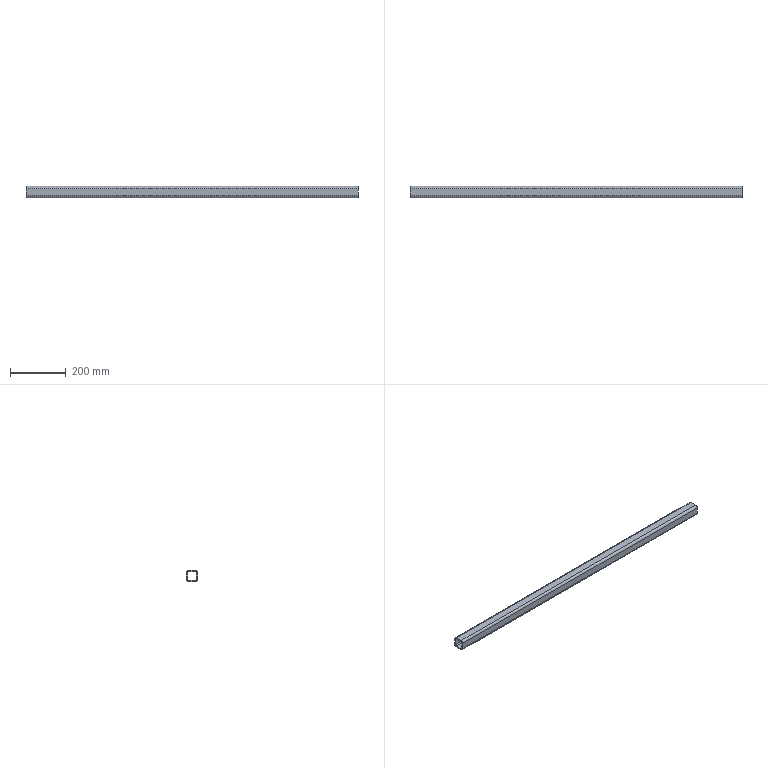Part | SolidWorks | features WeldMemberFeat 1, WeldmentFeature 1 | 1 solid | 18 faces | box 1192 x 40 x 40 mm | volume 637477 mm3 | plane 10 | cylinder 8 | commonest cylinder face diameters 8 x4 16 x4
STEP:
#1=CARTESIAN_POINT('',(-1000.,20.,12.));
#2=VERTEX_POINT('',#1);
#3=CARTESIAN_POINT('',(-1000.,12.,20.));
#4=VERTEX_POINT('',#3);
#5=CARTESIAN_POINT('',(-1000.,12.,12.));
#6=DIRECTION('',(1.,0.,0.));
#7=DIRECTION('',(0.,0.,-1.));
#8=AXIS2_PLACEMENT_3D('',#5,#6,#7);
#9=CIRCLE('',#8,8.);
#10=EDGE_CURVE('',#2,#4,#9,.T.);
#11=ORIENTED_EDGE('',*,*,#10,.T.);
#12=CARTESIAN_POINT('',(192.,12.,20.));
#13=VERTEX_POINT('',#12);
#14=CARTESIAN_POINT('',(192.,12.,20.));
#15=DIRECTION('',(-1.,0.,0.));
#16=VECTOR('',#15,1000.);
#17=LINE('',#14,#16);
#18=EDGE_CURVE('',#13,#4,#17,.T.);
#19=ORIENTED_EDGE('',*,*,#18,.F.);
#20=CARTESIAN_POINT('',(192.,20.,12.));
#21=VERTEX_POINT('',#20);
#22=CARTESIAN_POINT('',(192.,12.,12.));
#23=DIRECTION('',(1.,0.,0.));
#24=DIRECTION('',(0.,0.,-1.));
#25=AXIS2_PLACEMENT_3D('',#22,#23,#24);
#26=CIRCLE('',#25,8.);
#27=EDGE_CURVE('',#21,#13,#26,.T.);
#28=ORIENTED_EDGE('',*,*,#27,.F.);
#29=CARTESIAN_POINT('',(192.,20.,12.));
#30=DIRECTION('',(-1.,0.,0.));
#31=VECTOR('',#30,1000.);
#32=LINE('',#29,#31);
#33=EDGE_CURVE('',#21,#2,#32,.T.);
#34=ORIENTED_EDGE('',*,*,#33,.T.);
#35=EDGE_LOOP('',(#11,#19,#28,#34));
#36=FACE_OUTER_BOUND('',#35,.T.);
#37=CARTESIAN_POINT('',(192.,12.,12.));
#38=DIRECTION('',(-1.,0.,0.));
#39=DIRECTION('',(0.,0.,1.));
#40=AXIS2_PLACEMENT_3D('',#37,#38,#39);
#41=CYLINDRICAL_SURFACE('',#40,8.);
#42=ADVANCED_FACE('',(#36),#41,.T.);
#43=CARTESIAN_POINT('',(-1000.,-12.,20.));
#44=VERTEX_POINT('',#43);
#45=CARTESIAN_POINT('',(-1000.,12.,20.));
#46=DIRECTION('',(0.,-1.,0.));
#47=VECTOR('',#46,1000.);
#48=LINE('',#45,#47);
#49=EDGE_CURVE('',#4,#44,#48,.T.);
#50=ORIENTED_EDGE('',*,*,#49,.T.);
#51=CARTESIAN_POINT('',(192.,-12.,20.));
#52=VERTEX_POINT('',#51);
#53=CARTESIAN_POINT('',(192.,-12.,20.));
#54=DIRECTION('',(-1.,0.,0.));
#55=VECTOR('',#54,1000.);
#56=LINE('',#53,#55);
#57=EDGE_CURVE('',#52,#44,#56,.T.);
#58=ORIENTED_EDGE('',*,*,#57,.F.);
#59=CARTESIAN_POINT('',(192.,12.,20.));
#60=DIRECTION('',(0.,-1.,0.));
#61=VECTOR('',#60,1000.);
#62=LINE('',#59,#61);
#63=EDGE_CURVE('',#13,#52,#62,.T.);
#64=ORIENTED_EDGE('',*,*,#63,.F.);
#65=ORIENTED_EDGE('',*,*,#18,.T.);
#66=EDGE_LOOP('',(#50,#58,#64,#65));
#67=FACE_OUTER_BOUND('',#66,.T.);
#68=CARTESIAN_POINT('',(192.,12.,20.));
#69=DIRECTION('',(0.,0.,-1.));
#70=DIRECTION('',(-1.,0.,0.));
#71=AXIS2_PLACEMENT_3D('',#68,#69,#70);
#72=PLANE('',#71);
#73=ADVANCED_FACE('',(#67),#72,.F.);
#74=CARTESIAN_POINT('',(-1000.,-20.,12.));
#75=VERTEX_POINT('',#74);
#76=CARTESIAN_POINT('',(-1000.,-12.,12.));
#77=DIRECTION('',(1.,0.,0.));
#78=DIRECTION('',(0.,0.,-1.));
#79=AXIS2_PLACEMENT_3D('',#76,#77,#78);
#80=CIRCLE('',#79,8.);
#81=EDGE_CURVE('',#44,#75,#80,.T.);
#82=ORIENTED_EDGE('',*,*,#81,.T.);
#83=CARTESIAN_POINT('',(192.,-20.,12.));
#84=VERTEX_POINT('',#83);
#85=CARTESIAN_POINT('',(192.,-20.,12.));
#86=DIRECTION('',(-1.,0.,0.));
#87=VECTOR('',#86,1000.);
#88=LINE('',#85,#87);
#89=EDGE_CURVE('',#84,#75,#88,.T.);
#90=ORIENTED_EDGE('',*,*,#89,.F.);
#91=CARTESIAN_POINT('',(192.,-12.,12.));
#92=DIRECTION('',(1.,0.,0.));
#93=DIRECTION('',(0.,0.,-1.));
#94=AXIS2_PLACEMENT_3D('',#91,#92,#93);
#95=CIRCLE('',#94,8.);
#96=EDGE_CURVE('',#52,#84,#95,.T.);
#97=ORIENTED_EDGE('',*,*,#96,.F.);
#98=ORIENTED_EDGE('',*,*,#57,.T.);
#99=EDGE_LOOP('',(#82,#90,#97,#98));
#100=FACE_OUTER_BOUND('',#99,.T.);
#101=CARTESIAN_POINT('',(192.,-12.,12.));
#102=DIRECTION('',(-1.,0.,0.));
#103=DIRECTION('',(0.,0.,1.));
#104=AXIS2_PLACEMENT_3D('',#101,#102,#103);
#105=CYLINDRICAL_SURFACE('',#104,8.);
#106=ADVANCED_FACE('',(#100),#105,.T.);
#107=CARTESIAN_POINT('',(-1000.,-20.,-12.));
#108=VERTEX_POINT('',#107);
#109=CARTESIAN_POINT('',(-1000.,-20.,-12.));
#110=DIRECTION('',(0.,0.,-1.));
#111=VECTOR('',#110,1000.);
#112=LINE('',#109,#111);
#113=EDGE_CURVE('',#75,#108,#112,.T.);
#114=ORIENTED_EDGE('',*,*,#113,.T.);
#115=CARTESIAN_POINT('',(192.,-20.,-12.));
#116=VERTEX_POINT('',#115);
#117=CARTESIAN_POINT('',(192.,-20.,-12.));
#118=DIRECTION('',(-1.,0.,0.));
#119=VECTOR('',#118,1000.);
#120=LINE('',#117,#119);
#121=EDGE_CURVE('',#116,#108,#120,.T.);
#122=ORIENTED_EDGE('',*,*,#121,.F.);
#123=CARTESIAN_POINT('',(192.,-20.,-12.));
#124=DIRECTION('',(0.,0.,-1.));
#125=VECTOR('',#124,1000.);
#126=LINE('',#123,#125);
#127=EDGE_CURVE('',#84,#116,#126,.T.);
#128=ORIENTED_EDGE('',*,*,#127,.F.);
#129=ORIENTED_EDGE('',*,*,#89,.T.);
#130=EDGE_LOOP('',(#114,#122,#128,#129));
#131=FACE_OUTER_BOUND('',#130,.T.);
#132=CARTESIAN_POINT('',(192.,-20.,-12.));
#133=DIRECTION('',(0.,1.,0.));
#134=DIRECTION('',(0.,0.,1.));
#135=AXIS2_PLACEMENT_3D('',#132,#133,#134);
#136=PLANE('',#135);
#137=ADVANCED_FACE('',(#131),#136,.F.);
#138=CARTESIAN_POINT('',(-1000.,-12.,-20.));
#139=VERTEX_POINT('',#138);
#140=CARTESIAN_POINT('',(-1000.,-12.,-12.));
#141=DIRECTION('',(1.,0.,0.));
#142=DIRECTION('',(0.,0.,-1.));
#143=AXIS2_PLACEMENT_3D('',#140,#141,#142);
#144=CIRCLE('',#143,8.);
#145=EDGE_CURVE('',#108,#139,#144,.T.);
#146=ORIENTED_EDGE('',*,*,#145,.T.);
#147=CARTESIAN_POINT('',(192.,-12.,-20.));
#148=VERTEX_POINT('',#147);
#149=CARTESIAN_POINT('',(192.,-12.,-20.));
#150=DIRECTION('',(-1.,0.,0.));
#151=VECTOR('',#150,1000.);
#152=LINE('',#149,#151);
#153=EDGE_CURVE('',#148,#139,#152,.T.);
#154=ORIENTED_EDGE('',*,*,#153,.F.);
#155=CARTESIAN_POINT('',(192.,-12.,-12.));
#156=DIRECTION('',(1.,0.,0.));
#157=DIRECTION('',(0.,0.,-1.));
#158=AXIS2_PLACEMENT_3D('',#155,#156,#157);
#159=CIRCLE('',#158,8.);
#160=EDGE_CURVE('',#116,#148,#159,.T.);
#161=ORIENTED_EDGE('',*,*,#160,.F.);
#162=ORIENTED_EDGE('',*,*,#121,.T.);
#163=EDGE_LOOP('',(#146,#154,#161,#162));
#164=FACE_OUTER_BOUND('',#163,.T.);
#165=CARTESIAN_POINT('',(192.,-12.,-12.));
#166=DIRECTION('',(-1.,0.,0.));
#167=DIRECTION('',(0.,0.,1.));
#168=AXIS2_PLACEMENT_3D('',#165,#166,#167);
#169=CYLINDRICAL_SURFACE('',#168,8.);
#170=ADVANCED_FACE('',(#164),#169,.T.);
#171=CARTESIAN_POINT('',(-1000.,12.,-20.));
#172=VERTEX_POINT('',#171);
#173=CARTESIAN_POINT('',(-1000.,-12.,-20.));
#174=DIRECTION('',(0.,1.,0.));
#175=VECTOR('',#174,1000.);
#176=LINE('',#173,#175);
#177=EDGE_CURVE('',#139,#172,#176,.T.);
#178=ORIENTED_EDGE('',*,*,#177,.T.);
#179=CARTESIAN_POINT('',(192.,12.,-20.));
#180=VERTEX_POINT('',#179);
#181=CARTESIAN_POINT('',(192.,12.,-20.));
#182=DIRECTION('',(-1.,0.,0.));
#183=VECTOR('',#182,1000.);
#184=LINE('',#181,#183);
#185=EDGE_CURVE('',#180,#172,#184,.T.);
#186=ORIENTED_EDGE('',*,*,#185,.F.);
#187=CARTESIAN_POINT('',(192.,-12.,-20.));
#188=DIRECTION('',(0.,1.,0.));
#189=VECTOR('',#188,1000.);
#190=LINE('',#187,#189);
#191=EDGE_CURVE('',#148,#180,#190,.T.);
#192=ORIENTED_EDGE('',*,*,#191,.F.);
#193=ORIENTED_EDGE('',*,*,#153,.T.);
#194=EDGE_LOOP('',(#178,#186,#192,#193));
#195=FACE_OUTER_BOUND('',#194,.T.);
#196=CARTESIAN_POINT('',(192.,-12.,-20.));
#197=DIRECTION('',(0.,0.,1.));
#198=DIRECTION('',(1.,0.,0.));
#199=AXIS2_PLACEMENT_3D('',#196,#197,#198);
#200=PLANE('',#199);
#201=ADVANCED_FACE('',(#195),#200,.F.);
#202=CARTESIAN_POINT('',(-1000.,20.,-12.));
#203=VERTEX_POINT('',#202);
#204=CARTESIAN_POINT('',(-1000.,12.,-12.));
#205=DIRECTION('',(1.,0.,0.));
#206=DIRECTION('',(0.,0.,-1.));
#207=AXIS2_PLACEMENT_3D('',#204,#205,#206);
#208=CIRCLE('',#207,8.);
#209=EDGE_CURVE('',#172,#203,#208,.T.);
#210=ORIENTED_EDGE('',*,*,#209,.T.);
#211=CARTESIAN_POINT('',(192.,20.,-12.));
#212=VERTEX_POINT('',#211);
#213=CARTESIAN_POINT('',(192.,20.,-12.));
#214=DIRECTION('',(-1.,0.,0.));
#215=VECTOR('',#214,1000.);
#216=LINE('',#213,#215);
#217=EDGE_CURVE('',#212,#203,#216,.T.);
#218=ORIENTED_EDGE('',*,*,#217,.F.);
#219=CARTESIAN_POINT('',(192.,12.,-12.));
#220=DIRECTION('',(1.,0.,0.));
#221=DIRECTION('',(0.,0.,-1.));
#222=AXIS2_PLACEMENT_3D('',#219,#220,#221);
#223=CIRCLE('',#222,8.);
#224=EDGE_CURVE('',#180,#212,#223,.T.);
#225=ORIENTED_EDGE('',*,*,#224,.F.);
#226=ORIENTED_EDGE('',*,*,#185,.T.);
#227=EDGE_LOOP('',(#210,#218,#225,#226));
#228=FACE_OUTER_BOUND('',#227,.T.);
#229=CARTESIAN_POINT('',(192.,12.,-12.));
#230=DIRECTION('',(-1.,0.,0.));
#231=DIRECTION('',(0.,0.,1.));
#232=AXIS2_PLACEMENT_3D('',#229,#230,#231);
#233=CYLINDRICAL_SURFACE('',#232,8.);
#234=ADVANCED_FACE('',(#228),#233,.T.);
#235=CARTESIAN_POINT('',(-1000.,-12.,16.));
#236=VERTEX_POINT('',#235);
#237=CARTESIAN_POINT('',(-1000.,-16.,12.));
#238=VERTEX_POINT('',#237);
#239=CARTESIAN_POINT('',(-1000.,-12.,12.));
#240=DIRECTION('',(1.,0.,0.));
#241=DIRECTION('',(0.,0.,-1.));
#242=AXIS2_PLACEMENT_3D('',#239,#240,#241);
#243=CIRCLE('',#242,4.);
#244=EDGE_CURVE('',#236,#238,#243,.T.);
#245=ORIENTED_EDGE('',*,*,#244,.F.);
#246=CARTESIAN_POINT('',(192.,-12.,16.));
#247=VERTEX_POINT('',#246);
#248=CARTESIAN_POINT('',(192.,-12.,16.));
#249=DIRECTION('',(-1.,0.,0.));
#250=VECTOR('',#249,1000.);
#251=LINE('',#248,#250);
#252=EDGE_CURVE('',#247,#236,#251,.T.);
#253=ORIENTED_EDGE('',*,*,#252,.F.);
#254=CARTESIAN_POINT('',(192.,-16.,12.));
#255=VERTEX_POINT('',#254);
#256=CARTESIAN_POINT('',(192.,-12.,12.));
#257=DIRECTION('',(1.,0.,0.));
#258=DIRECTION('',(0.,0.,-1.));
#259=AXIS2_PLACEMENT_3D('',#256,#257,#258);
#260=CIRCLE('',#259,4.);
#261=EDGE_CURVE('',#247,#255,#260,.T.);
#262=ORIENTED_EDGE('',*,*,#261,.T.);
#263=CARTESIAN_POINT('',(192.,-16.,12.));
#264=DIRECTION('',(-1.,0.,0.));
#265=VECTOR('',#264,1000.);
#266=LINE('',#263,#265);
#267=EDGE_CURVE('',#255,#238,#266,.T.);
#268=ORIENTED_EDGE('',*,*,#267,.T.);
#269=EDGE_LOOP('',(#245,#253,#262,#268));
#270=FACE_OUTER_BOUND('',#269,.T.);
#271=CARTESIAN_POINT('',(192.,-12.,12.));
#272=DIRECTION('',(-1.,0.,0.));
#273=DIRECTION('',(0.,0.,1.));
#274=AXIS2_PLACEMENT_3D('',#271,#272,#273);
#275=CYLINDRICAL_SURFACE('',#274,4.);
#276=ADVANCED_FACE('',(#270),#275,.F.);
#277=CARTESIAN_POINT('',(-1000.,12.,16.));
#278=VERTEX_POINT('',#277);
#279=CARTESIAN_POINT('',(-1000.,12.,16.));
#280=DIRECTION('',(0.,-1.,0.));
#281=VECTOR('',#280,1000.);
#282=LINE('',#279,#281);
#283=EDGE_CURVE('',#278,#236,#282,.T.);
#284=ORIENTED_EDGE('',*,*,#283,.F.);
#285=CARTESIAN_POINT('',(192.,12.,16.));
#286=VERTEX_POINT('',#285);
#287=CARTESIAN_POINT('',(192.,12.,16.));
#288=DIRECTION('',(-1.,0.,0.));
#289=VECTOR('',#288,1000.);
#290=LINE('',#287,#289);
#291=EDGE_CURVE('',#286,#278,#290,.T.);
#292=ORIENTED_EDGE('',*,*,#291,.F.);
#293=CARTESIAN_POINT('',(192.,12.,16.));
#294=DIRECTION('',(0.,-1.,0.));
#295=VECTOR('',#294,1000.);
#296=LINE('',#293,#295);
#297=EDGE_CURVE('',#286,#247,#296,.T.);
#298=ORIENTED_EDGE('',*,*,#297,.T.);
#299=ORIENTED_EDGE('',*,*,#252,.T.);
#300=EDGE_LOOP('',(#284,#292,#298,#299));
#301=FACE_OUTER_BOUND('',#300,.T.);
#302=CARTESIAN_POINT('',(192.,12.,16.));
#303=DIRECTION('',(0.,0.,-1.));
#304=DIRECTION('',(-1.,0.,0.));
#305=AXIS2_PLACEMENT_3D('',#302,#303,#304);
#306=PLANE('',#305);
#307=ADVANCED_FACE('',(#301),#306,.T.);
#308=CARTESIAN_POINT('',(-1000.,16.,12.));
#309=VERTEX_POINT('',#308);
#310=CARTESIAN_POINT('',(-1000.,12.,12.));
#311=DIRECTION('',(1.,0.,0.));
#312=DIRECTION('',(0.,0.,-1.));
#313=AXIS2_PLACEMENT_3D('',#310,#311,#312);
#314=CIRCLE('',#313,4.);
#315=EDGE_CURVE('',#309,#278,#314,.T.);
#316=ORIENTED_EDGE('',*,*,#315,.F.);
#317=CARTESIAN_POINT('',(192.,16.,12.));
#318=VERTEX_POINT('',#317);
#319=CARTESIAN_POINT('',(192.,16.,12.));
#320=DIRECTION('',(-1.,0.,0.));
#321=VECTOR('',#320,1000.);
#322=LINE('',#319,#321);
#323=EDGE_CURVE('',#318,#309,#322,.T.);
#324=ORIENTED_EDGE('',*,*,#323,.F.);
#325=CARTESIAN_POINT('',(192.,12.,12.));
#326=DIRECTION('',(1.,0.,0.));
#327=DIRECTION('',(0.,0.,-1.));
#328=AXIS2_PLACEMENT_3D('',#325,#326,#327);
#329=CIRCLE('',#328,4.);
#330=EDGE_CURVE('',#318,#286,#329,.T.);
#331=ORIENTED_EDGE('',*,*,#330,.T.);
#332=ORIENTED_EDGE('',*,*,#291,.T.);
#333=EDGE_LOOP('',(#316,#324,#331,#332));
#334=FACE_OUTER_BOUND('',#333,.T.);
#335=CARTESIAN_POINT('',(192.,12.,12.));
#336=DIRECTION('',(-1.,0.,0.));
#337=DIRECTION('',(0.,0.,1.));
#338=AXIS2_PLACEMENT_3D('',#335,#336,#337);
#339=CYLINDRICAL_SURFACE('',#338,4.);
#340=ADVANCED_FACE('',(#334),#339,.F.);
#341=CARTESIAN_POINT('',(-1000.,16.,-12.));
#342=VERTEX_POINT('',#341);
#343=CARTESIAN_POINT('',(-1000.,16.,12.));
#344=DIRECTION('',(0.,0.,1.));
#345=VECTOR('',#344,1000.);
#346=LINE('',#343,#345);
#347=EDGE_CURVE('',#342,#309,#346,.T.);
#348=ORIENTED_EDGE('',*,*,#347,.F.);
#349=CARTESIAN_POINT('',(192.,16.,-12.));
#350=VERTEX_POINT('',#349);
#351=CARTESIAN_POINT('',(192.,16.,-12.));
#352=DIRECTION('',(-1.,0.,0.));
#353=VECTOR('',#352,1000.);
#354=LINE('',#351,#353);
#355=EDGE_CURVE('',#350,#342,#354,.T.);
#356=ORIENTED_EDGE('',*,*,#355,.F.);
#357=CARTESIAN_POINT('',(192.,16.,12.));
#358=DIRECTION('',(0.,0.,1.));
#359=VECTOR('',#358,1000.);
#360=LINE('',#357,#359);
#361=EDGE_CURVE('',#350,#318,#360,.T.);
#362=ORIENTED_EDGE('',*,*,#361,.T.);
#363=ORIENTED_EDGE('',*,*,#323,.T.);
#364=EDGE_LOOP('',(#348,#356,#362,#363));
#365=FACE_OUTER_BOUND('',#364,.T.);
#366=CARTESIAN_POINT('',(192.,16.,12.));
#367=DIRECTION('',(0.,-1.,0.));
#368=DIRECTION('',(0.,0.,-1.));
#369=AXIS2_PLACEMENT_3D('',#366,#367,#368);
#370=PLANE('',#369);
#371=ADVANCED_FACE('',(#365),#370,.T.);
#372=CARTESIAN_POINT('',(-1000.,12.,-16.));
#373=VERTEX_POINT('',#372);
#374=CARTESIAN_POINT('',(-1000.,12.,-12.));
#375=DIRECTION('',(1.,0.,0.));
#376=DIRECTION('',(0.,0.,-1.));
#377=AXIS2_PLACEMENT_3D('',#374,#375,#376);
#378=CIRCLE('',#377,4.);
#379=EDGE_CURVE('',#373,#342,#378,.T.);
#380=ORIENTED_EDGE('',*,*,#379,.F.);
#381=CARTESIAN_POINT('',(192.,12.,-16.));
#382=VERTEX_POINT('',#381);
#383=CARTESIAN_POINT('',(192.,12.,-16.));
#384=DIRECTION('',(-1.,0.,0.));
#385=VECTOR('',#384,1000.);
#386=LINE('',#383,#385);
#387=EDGE_CURVE('',#382,#373,#386,.T.);
#388=ORIENTED_EDGE('',*,*,#387,.F.);
#389=CARTESIAN_POINT('',(192.,12.,-12.));
#390=DIRECTION('',(1.,0.,0.));
#391=DIRECTION('',(0.,0.,-1.));
#392=AXIS2_PLACEMENT_3D('',#389,#390,#391);
#393=CIRCLE('',#392,4.);
#394=EDGE_CURVE('',#382,#350,#393,.T.);
#395=ORIENTED_EDGE('',*,*,#394,.T.);
#396=ORIENTED_EDGE('',*,*,#355,.T.);
#397=EDGE_LOOP('',(#380,#388,#395,#396));
#398=FACE_OUTER_BOUND('',#397,.T.);
#399=CARTESIAN_POINT('',(192.,12.,-12.));
#400=DIRECTION('',(-1.,0.,0.));
#401=DIRECTION('',(0.,0.,1.));
#402=AXIS2_PLACEMENT_3D('',#399,#400,#401);
#403=CYLINDRICAL_SURFACE('',#402,4.);
#404=ADVANCED_FACE('',(#398),#403,.F.);
#405=CARTESIAN_POINT('',(-1000.,-12.,-16.));
#406=VERTEX_POINT('',#405);
#407=CARTESIAN_POINT('',(-1000.,-12.,-16.));
#408=DIRECTION('',(0.,1.,0.));
#409=VECTOR('',#408,1000.);
#410=LINE('',#407,#409);
#411=EDGE_CURVE('',#406,#373,#410,.T.);
#412=ORIENTED_EDGE('',*,*,#411,.F.);
#413=CARTESIAN_POINT('',(192.,-12.,-16.));
#414=VERTEX_POINT('',#413);
#415=CARTESIAN_POINT('',(192.,-12.,-16.));
#416=DIRECTION('',(-1.,0.,0.));
#417=VECTOR('',#416,1000.);
#418=LINE('',#415,#417);
#419=EDGE_CURVE('',#414,#406,#418,.T.);
#420=ORIENTED_EDGE('',*,*,#419,.F.);
#421=CARTESIAN_POINT('',(192.,-12.,-16.));
#422=DIRECTION('',(0.,1.,0.));
#423=VECTOR('',#422,1000.);
#424=LINE('',#421,#423);
#425=EDGE_CURVE('',#414,#382,#424,.T.);
#426=ORIENTED_EDGE('',*,*,#425,.T.);
#427=ORIENTED_EDGE('',*,*,#387,.T.);
#428=EDGE_LOOP('',(#412,#420,#426,#427));
#429=FACE_OUTER_BOUND('',#428,.T.);
#430=CARTESIAN_POINT('',(192.,-12.,-16.));
#431=DIRECTION('',(0.,0.,1.));
#432=DIRECTION('',(1.,0.,0.));
#433=AXIS2_PLACEMENT_3D('',#430,#431,#432);
#434=PLANE('',#433);
#435=ADVANCED_FACE('',(#429),#434,.T.);
#436=CARTESIAN_POINT('',(-1000.,-16.,-12.));
#437=VERTEX_POINT('',#436);
#438=CARTESIAN_POINT('',(-1000.,-12.,-12.));
#439=DIRECTION('',(1.,0.,0.));
#440=DIRECTION('',(0.,0.,-1.));
#441=AXIS2_PLACEMENT_3D('',#438,#439,#440);
#442=CIRCLE('',#441,4.);
#443=EDGE_CURVE('',#437,#406,#442,.T.);
#444=ORIENTED_EDGE('',*,*,#443,.F.);
#445=CARTESIAN_POINT('',(192.,-16.,-12.));
#446=VERTEX_POINT('',#445);
#447=CARTESIAN_POINT('',(192.,-16.,-12.));
#448=DIRECTION('',(-1.,0.,0.));
#449=VECTOR('',#448,1000.);
#450=LINE('',#447,#449);
#451=EDGE_CURVE('',#446,#437,#450,.T.);
#452=ORIENTED_EDGE('',*,*,#451,.F.);
#453=CARTESIAN_POINT('',(192.,-12.,-12.));
#454=DIRECTION('',(1.,0.,0.));
#455=DIRECTION('',(0.,0.,-1.));
#456=AXIS2_PLACEMENT_3D('',#453,#454,#455);
#457=CIRCLE('',#456,4.);
#458=EDGE_CURVE('',#446,#414,#457,.T.);
#459=ORIENTED_EDGE('',*,*,#458,.T.);
#460=ORIENTED_EDGE('',*,*,#419,.T.);
#461=EDGE_LOOP('',(#444,#452,#459,#460));
#462=FACE_OUTER_BOUND('',#461,.T.);
#463=CARTESIAN_POINT('',(192.,-12.,-12.));
#464=DIRECTION('',(-1.,0.,0.));
#465=DIRECTION('',(0.,0.,1.));
#466=AXIS2_PLACEMENT_3D('',#463,#464,#465);
#467=CYLINDRICAL_SURFACE('',#466,4.);
#468=ADVANCED_FACE('',(#462),#467,.F.);
#469=CARTESIAN_POINT('',(-1000.,-16.,-12.));
#470=DIRECTION('',(0.,0.,-1.));
#471=VECTOR('',#470,1000.);
#472=LINE('',#469,#471);
#473=EDGE_CURVE('',#238,#437,#472,.T.);
#474=ORIENTED_EDGE('',*,*,#473,.F.);
#475=ORIENTED_EDGE('',*,*,#267,.F.);
#476=CARTESIAN_POINT('',(192.,-16.,-12.));
#477=DIRECTION('',(0.,0.,-1.));
#478=VECTOR('',#477,1000.);
#479=LINE('',#476,#478);
#480=EDGE_CURVE('',#255,#446,#479,.T.);
#481=ORIENTED_EDGE('',*,*,#480,.T.);
#482=ORIENTED_EDGE('',*,*,#451,.T.);
#483=EDGE_LOOP('',(#474,#475,#481,#482));
#484=FACE_OUTER_BOUND('',#483,.T.);
#485=CARTESIAN_POINT('',(192.,-16.,-12.));
#486=DIRECTION('',(0.,1.,0.));
#487=DIRECTION('',(0.,0.,1.));
#488=AXIS2_PLACEMENT_3D('',#485,#486,#487);
#489=PLANE('',#488);
#490=ADVANCED_FACE('',(#484),#489,.T.);
#491=CARTESIAN_POINT('',(-1000.,20.,12.));
#492=DIRECTION('',(0.,0.,1.));
#493=VECTOR('',#492,1000.);
#494=LINE('',#491,#493);
#495=EDGE_CURVE('',#203,#2,#494,.T.);
#496=ORIENTED_EDGE('',*,*,#495,.T.);
#497=ORIENTED_EDGE('',*,*,#33,.F.);
#498=CARTESIAN_POINT('',(192.,20.,12.));
#499=DIRECTION('',(0.,0.,1.));
#500=VECTOR('',#499,1000.);
#501=LINE('',#498,#500);
#502=EDGE_CURVE('',#212,#21,#501,.T.);
#503=ORIENTED_EDGE('',*,*,#502,.F.);
#504=ORIENTED_EDGE('',*,*,#217,.T.);
#505=EDGE_LOOP('',(#496,#497,#503,#504));
#506=FACE_OUTER_BOUND('',#505,.T.);
#507=CARTESIAN_POINT('',(192.,20.,12.));
#508=DIRECTION('',(0.,-1.,0.));
#509=DIRECTION('',(0.,0.,-1.));
#510=AXIS2_PLACEMENT_3D('',#507,#508,#509);
#511=PLANE('',#510);
#512=ADVANCED_FACE('',(#506),#511,.F.);
#513=ORIENTED_EDGE('',*,*,#261,.F.);
#514=ORIENTED_EDGE('',*,*,#297,.F.);
#515=ORIENTED_EDGE('',*,*,#330,.F.);
#516=ORIENTED_EDGE('',*,*,#361,.F.);
#517=ORIENTED_EDGE('',*,*,#394,.F.);
#518=ORIENTED_EDGE('',*,*,#425,.F.);
#519=ORIENTED_EDGE('',*,*,#458,.F.);
#520=ORIENTED_EDGE('',*,*,#480,.F.);
#521=EDGE_LOOP('',(#513,#514,#515,#516,#517,#518,#519,#520));
#522=FACE_BOUND('',#521,.T.);
#523=ORIENTED_EDGE('',*,*,#27,.T.);
#524=ORIENTED_EDGE('',*,*,#63,.T.);
#525=ORIENTED_EDGE('',*,*,#96,.T.);
#526=ORIENTED_EDGE('',*,*,#127,.T.);
#527=ORIENTED_EDGE('',*,*,#160,.T.);
#528=ORIENTED_EDGE('',*,*,#191,.T.);
#529=ORIENTED_EDGE('',*,*,#224,.T.);
#530=ORIENTED_EDGE('',*,*,#502,.T.);
#531=EDGE_LOOP('',(#523,#524,#525,#526,#527,#528,#529,#530));
#532=FACE_OUTER_BOUND('',#531,.T.);
#533=CARTESIAN_POINT('',(192.,12.,12.));
#534=DIRECTION('',(1.,0.,0.));
#535=DIRECTION('',(0.,0.,-1.));
#536=AXIS2_PLACEMENT_3D('',#533,#534,#535);
#537=PLANE('',#536);
#538=ADVANCED_FACE('',(#522,#532),#537,.T.);
#539=ORIENTED_EDGE('',*,*,#244,.T.);
#540=ORIENTED_EDGE('',*,*,#473,.T.);
#541=ORIENTED_EDGE('',*,*,#443,.T.);
#542=ORIENTED_EDGE('',*,*,#411,.T.);
#543=ORIENTED_EDGE('',*,*,#379,.T.);
#544=ORIENTED_EDGE('',*,*,#347,.T.);
#545=ORIENTED_EDGE('',*,*,#315,.T.);
#546=ORIENTED_EDGE('',*,*,#283,.T.);
#547=EDGE_LOOP('',(#539,#540,#541,#542,#543,#544,#545,#546));
#548=FACE_BOUND('',#547,.T.);
#549=ORIENTED_EDGE('',*,*,#10,.F.);
#550=ORIENTED_EDGE('',*,*,#495,.F.);
#551=ORIENTED_EDGE('',*,*,#209,.F.);
#552=ORIENTED_EDGE('',*,*,#177,.F.);
#553=ORIENTED_EDGE('',*,*,#145,.F.);
#554=ORIENTED_EDGE('',*,*,#113,.F.);
#555=ORIENTED_EDGE('',*,*,#81,.F.);
#556=ORIENTED_EDGE('',*,*,#49,.F.);
#557=EDGE_LOOP('',(#549,#550,#551,#552,#553,#554,#555,#556));
#558=FACE_OUTER_BOUND('',#557,.T.);
#559=CARTESIAN_POINT('',(-1000.,12.,12.));
#560=DIRECTION('',(1.,0.,0.));
#561=DIRECTION('',(0.,0.,-1.));
#562=AXIS2_PLACEMENT_3D('',#559,#560,#561);
#563=PLANE('',#562);
#564=ADVANCED_FACE('',(#548,#558),#563,.F.);
#565=CLOSED_SHELL('',(#42,#73,#106,#137,#170,#201,#234,#276,#307,#340,#371,#404,#435,#468,#490,#512,#538,#564));
#566=MANIFOLD_SOLID_BREP('',#565);
#567=CARTESIAN_POINT('',(0.,0.,0.));
#568=DIRECTION('',(0.,0.,1.));
#569=DIRECTION('',(1.,0.,0.));
#570=AXIS2_PLACEMENT_3D('',#567,#568,#569);
#571=(LENGTH_UNIT()NAMED_UNIT(*)SI_UNIT(.MILLI.,.METRE.));
#572=UNCERTAINTY_MEASURE_WITH_UNIT(LENGTH_MEASURE(0.00001),#571,'','');
#573=(NAMED_UNIT(*)PLANE_ANGLE_UNIT()SI_UNIT($,.RADIAN.));
#574=(NAMED_UNIT(*)SI_UNIT($,.STERADIAN.)SOLID_ANGLE_UNIT());
#575=(GEOMETRIC_REPRESENTATION_CONTEXT(3)GLOBAL_UNCERTAINTY_ASSIGNED_CONTEXT((#572))GLOBAL_UNIT_ASSIGNED_CONTEXT((#571,#573,#574))REPRESENTATION_CONTEXT('',''));
#576=ADVANCED_BREP_SHAPE_REPRESENTATION('',(#566,#570),#575);